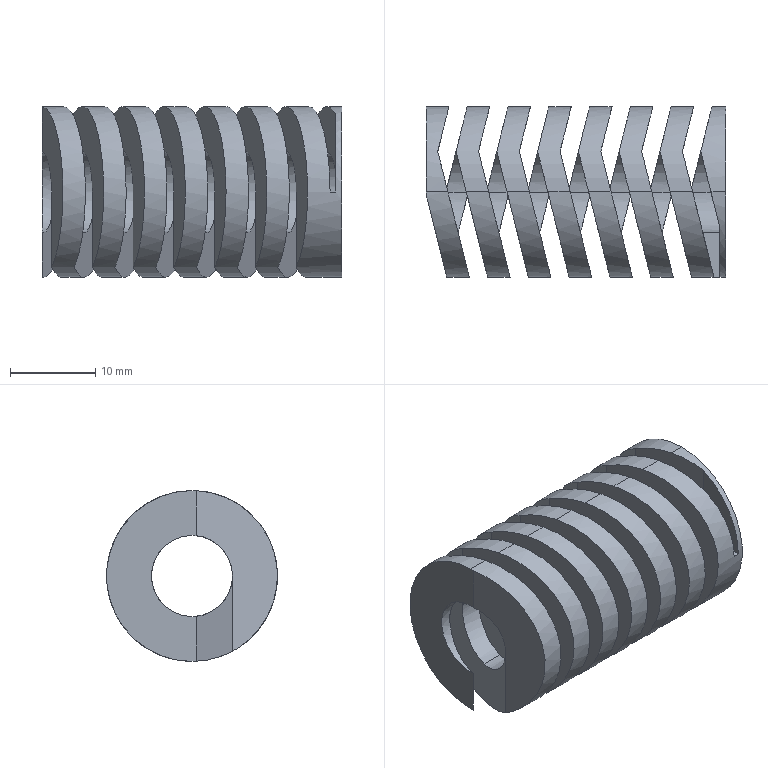Part | SolidWorks | features BaseBody 1 | 1 solid | 66 faces | box 35 x 20 x 20 mm | volume 4844 mm3 | plane 34 | cylinder 32 | commonest cylinder face diameters 9.5 x16 20 x16